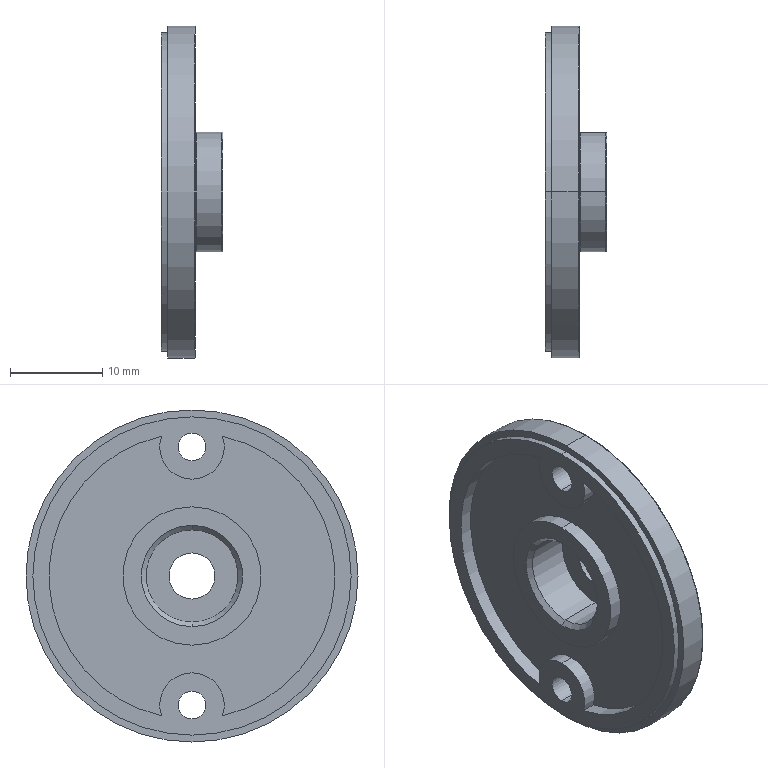Part | SolidWorks | features BaseBody 1 | 1 solid | 38 faces | box 6.7 x 36 x 36 mm | volume 2836 mm3 | cylinder 21 | plane 7 | torus 6 | cone 4 | commonest cylinder face diameters 3 x4 7 x3 5 x2 10 x2 13 x2 15 x2
STEP:
#1=CARTESIAN_POINT('',(1.5,0.,7.5));
#2=VERTEX_POINT('',#1);
#3=CARTESIAN_POINT('',(1.5,0.,-7.5));
#4=VERTEX_POINT('',#3);
#5=CARTESIAN_POINT('',(1.5,0.,0.));
#6=DIRECTION('',(-1.,0.,0.));
#7=DIRECTION('',(0.,0.,1.));
#8=AXIS2_PLACEMENT_3D('',#5,#6,#7);
#9=CIRCLE('',#8,7.5);
#10=EDGE_CURVE('',#2,#4,#9,.T.);
#11=ORIENTED_EDGE('',*,*,#10,.F.);
#12=CARTESIAN_POINT('',(1.5,0.,0.));
#13=DIRECTION('',(-1.,0.,0.));
#14=DIRECTION('',(0.,0.,1.));
#15=AXIS2_PLACEMENT_3D('',#12,#13,#14);
#16=CIRCLE('',#15,7.5);
#17=EDGE_CURVE('',#4,#2,#16,.T.);
#18=ORIENTED_EDGE('',*,*,#17,.F.);
#19=EDGE_LOOP('',(#11,#18));
#20=FACE_BOUND('',#19,.T.);
#21=CARTESIAN_POINT('',(1.5,3.308,15.143));
#22=VERTEX_POINT('',#21);
#23=CARTESIAN_POINT('',(1.5,-3.308,15.143));
#24=VERTEX_POINT('',#23);
#25=CARTESIAN_POINT('',(1.5,0.,14.));
#26=DIRECTION('',(-1.,0.,0.));
#27=DIRECTION('',(0.,0.,1.));
#28=AXIS2_PLACEMENT_3D('',#25,#26,#27);
#29=CIRCLE('',#28,3.5);
#30=EDGE_CURVE('',#22,#24,#29,.T.);
#31=ORIENTED_EDGE('',*,*,#30,.F.);
#32=CARTESIAN_POINT('',(1.5,3.308,-15.143));
#33=VERTEX_POINT('',#32);
#34=CARTESIAN_POINT('',(1.5,0.,0.));
#35=DIRECTION('',(-1.,0.,0.));
#36=DIRECTION('',(0.,0.,1.));
#37=AXIS2_PLACEMENT_3D('',#34,#35,#36);
#38=CIRCLE('',#37,15.5);
#39=EDGE_CURVE('',#22,#33,#38,.T.);
#40=ORIENTED_EDGE('',*,*,#39,.T.);
#41=CARTESIAN_POINT('',(1.5,0.,-10.5));
#42=VERTEX_POINT('',#41);
#43=CARTESIAN_POINT('',(1.5,0.,-14.));
#44=DIRECTION('',(-1.,0.,0.));
#45=DIRECTION('',(0.,0.,1.));
#46=AXIS2_PLACEMENT_3D('',#43,#44,#45);
#47=CIRCLE('',#46,3.5);
#48=EDGE_CURVE('',#42,#33,#47,.T.);
#49=ORIENTED_EDGE('',*,*,#48,.F.);
#50=CARTESIAN_POINT('',(1.5,-3.308,-15.143));
#51=VERTEX_POINT('',#50);
#52=CARTESIAN_POINT('',(1.5,0.,-14.));
#53=DIRECTION('',(-1.,0.,0.));
#54=DIRECTION('',(0.,0.,1.));
#55=AXIS2_PLACEMENT_3D('',#52,#53,#54);
#56=CIRCLE('',#55,3.5);
#57=EDGE_CURVE('',#51,#42,#56,.T.);
#58=ORIENTED_EDGE('',*,*,#57,.F.);
#59=CARTESIAN_POINT('',(1.5,0.,0.));
#60=DIRECTION('',(-1.,0.,0.));
#61=DIRECTION('',(0.,0.,1.));
#62=AXIS2_PLACEMENT_3D('',#59,#60,#61);
#63=CIRCLE('',#62,15.5);
#64=EDGE_CURVE('',#51,#24,#63,.T.);
#65=ORIENTED_EDGE('',*,*,#64,.T.);
#66=EDGE_LOOP('',(#31,#40,#49,#58,#65));
#67=FACE_OUTER_BOUND('',#66,.T.);
#68=CARTESIAN_POINT('',(1.5,0.,0.));
#69=DIRECTION('',(-1.,0.,0.));
#70=DIRECTION('',(0.,0.,1.));
#71=AXIS2_PLACEMENT_3D('',#68,#69,#70);
#72=PLANE('',#71);
#73=ADVANCED_FACE('',(#20,#67),#72,.T.);
#74=CARTESIAN_POINT('',(0.,3.308,15.143));
#75=VERTEX_POINT('',#74);
#76=CARTESIAN_POINT('',(0.,3.308,-15.143));
#77=VERTEX_POINT('',#76);
#78=CARTESIAN_POINT('',(0.,0.,0.));
#79=DIRECTION('',(-1.,0.,0.));
#80=DIRECTION('',(0.,0.,1.));
#81=AXIS2_PLACEMENT_3D('',#78,#79,#80);
#82=CIRCLE('',#81,15.5);
#83=EDGE_CURVE('',#75,#77,#82,.T.);
#84=ORIENTED_EDGE('',*,*,#83,.T.);
#85=CARTESIAN_POINT('',(1.5,3.308,-15.143));
#86=DIRECTION('',(-1.,0.,0.));
#87=VECTOR('',#86,1000.);
#88=LINE('',#85,#87);
#89=EDGE_CURVE('',#33,#77,#88,.T.);
#90=ORIENTED_EDGE('',*,*,#89,.F.);
#91=ORIENTED_EDGE('',*,*,#39,.F.);
#92=CARTESIAN_POINT('',(1.5,3.308,15.143));
#93=DIRECTION('',(-1.,0.,0.));
#94=VECTOR('',#93,1000.);
#95=LINE('',#92,#94);
#96=EDGE_CURVE('',#22,#75,#95,.T.);
#97=ORIENTED_EDGE('',*,*,#96,.T.);
#98=EDGE_LOOP('',(#84,#90,#91,#97));
#99=FACE_OUTER_BOUND('',#98,.T.);
#100=CARTESIAN_POINT('',(1.5,0.,0.));
#101=DIRECTION('',(-1.,0.,0.));
#102=DIRECTION('',(0.,0.,1.));
#103=AXIS2_PLACEMENT_3D('',#100,#101,#102);
#104=CYLINDRICAL_SURFACE('',#103,15.5);
#105=ADVANCED_FACE('',(#99),#104,.F.);
#106=CARTESIAN_POINT('',(0.,0.,-7.5));
#107=VERTEX_POINT('',#106);
#108=CARTESIAN_POINT('',(1.5,0.,-7.5));
#109=DIRECTION('',(-1.,0.,0.));
#110=VECTOR('',#109,1000.);
#111=LINE('',#108,#110);
#112=EDGE_CURVE('',#4,#107,#111,.T.);
#113=ORIENTED_EDGE('',*,*,#112,.F.);
#114=ORIENTED_EDGE('',*,*,#17,.T.);
#115=CARTESIAN_POINT('',(0.,0.,7.5));
#116=VERTEX_POINT('',#115);
#117=CARTESIAN_POINT('',(1.5,0.,7.5));
#118=DIRECTION('',(-1.,0.,0.));
#119=VECTOR('',#118,1000.);
#120=LINE('',#117,#119);
#121=EDGE_CURVE('',#2,#116,#120,.T.);
#122=ORIENTED_EDGE('',*,*,#121,.T.);
#123=CARTESIAN_POINT('',(0.,0.,0.));
#124=DIRECTION('',(-1.,0.,0.));
#125=DIRECTION('',(0.,0.,1.));
#126=AXIS2_PLACEMENT_3D('',#123,#124,#125);
#127=CIRCLE('',#126,7.5);
#128=EDGE_CURVE('',#107,#116,#127,.T.);
#129=ORIENTED_EDGE('',*,*,#128,.F.);
#130=EDGE_LOOP('',(#113,#114,#122,#129));
#131=FACE_OUTER_BOUND('',#130,.T.);
#132=CARTESIAN_POINT('',(1.5,0.,0.));
#133=DIRECTION('',(-1.,0.,0.));
#134=DIRECTION('',(0.,0.,1.));
#135=AXIS2_PLACEMENT_3D('',#132,#133,#134);
#136=CYLINDRICAL_SURFACE('',#135,7.5);
#137=ADVANCED_FACE('',(#131),#136,.T.);
#138=CARTESIAN_POINT('',(0.,0.,-10.5));
#139=VERTEX_POINT('',#138);
#140=CARTESIAN_POINT('',(1.5,0.,-10.5));
#141=DIRECTION('',(-1.,0.,0.));
#142=VECTOR('',#141,1000.);
#143=LINE('',#140,#142);
#144=EDGE_CURVE('',#42,#139,#143,.T.);
#145=ORIENTED_EDGE('',*,*,#144,.F.);
#146=ORIENTED_EDGE('',*,*,#48,.T.);
#147=ORIENTED_EDGE('',*,*,#89,.T.);
#148=CARTESIAN_POINT('',(0.,0.,-14.));
#149=DIRECTION('',(-1.,0.,0.));
#150=DIRECTION('',(0.,0.,1.));
#151=AXIS2_PLACEMENT_3D('',#148,#149,#150);
#152=CIRCLE('',#151,3.5);
#153=EDGE_CURVE('',#139,#77,#152,.T.);
#154=ORIENTED_EDGE('',*,*,#153,.F.);
#155=EDGE_LOOP('',(#145,#146,#147,#154));
#156=FACE_OUTER_BOUND('',#155,.T.);
#157=CARTESIAN_POINT('',(1.5,0.,-14.));
#158=DIRECTION('',(-1.,0.,0.));
#159=DIRECTION('',(0.,0.,1.));
#160=AXIS2_PLACEMENT_3D('',#157,#158,#159);
#161=CYLINDRICAL_SURFACE('',#160,3.5);
#162=ADVANCED_FACE('',(#156),#161,.T.);
#163=CARTESIAN_POINT('',(0.,-3.308,-15.143));
#164=VERTEX_POINT('',#163);
#165=CARTESIAN_POINT('',(0.,-3.308,15.143));
#166=VERTEX_POINT('',#165);
#167=CARTESIAN_POINT('',(0.,0.,0.));
#168=DIRECTION('',(-1.,0.,0.));
#169=DIRECTION('',(0.,0.,1.));
#170=AXIS2_PLACEMENT_3D('',#167,#168,#169);
#171=CIRCLE('',#170,15.5);
#172=EDGE_CURVE('',#164,#166,#171,.T.);
#173=ORIENTED_EDGE('',*,*,#172,.T.);
#174=CARTESIAN_POINT('',(1.5,-3.308,15.143));
#175=DIRECTION('',(-1.,0.,0.));
#176=VECTOR('',#175,1000.);
#177=LINE('',#174,#176);
#178=EDGE_CURVE('',#24,#166,#177,.T.);
#179=ORIENTED_EDGE('',*,*,#178,.F.);
#180=ORIENTED_EDGE('',*,*,#64,.F.);
#181=CARTESIAN_POINT('',(1.5,-3.308,-15.143));
#182=DIRECTION('',(-1.,0.,0.));
#183=VECTOR('',#182,1000.);
#184=LINE('',#181,#183);
#185=EDGE_CURVE('',#51,#164,#184,.T.);
#186=ORIENTED_EDGE('',*,*,#185,.T.);
#187=EDGE_LOOP('',(#173,#179,#180,#186));
#188=FACE_OUTER_BOUND('',#187,.T.);
#189=CARTESIAN_POINT('',(1.5,0.,0.));
#190=DIRECTION('',(-1.,0.,0.));
#191=DIRECTION('',(0.,0.,1.));
#192=AXIS2_PLACEMENT_3D('',#189,#190,#191);
#193=CYLINDRICAL_SURFACE('',#192,15.5);
#194=ADVANCED_FACE('',(#188),#193,.F.);
#195=CARTESIAN_POINT('',(0.,0.,14.));
#196=DIRECTION('',(-1.,0.,0.));
#197=DIRECTION('',(0.,0.,1.));
#198=AXIS2_PLACEMENT_3D('',#195,#196,#197);
#199=CIRCLE('',#198,3.5);
#200=EDGE_CURVE('',#75,#166,#199,.T.);
#201=ORIENTED_EDGE('',*,*,#200,.F.);
#202=ORIENTED_EDGE('',*,*,#96,.F.);
#203=ORIENTED_EDGE('',*,*,#30,.T.);
#204=ORIENTED_EDGE('',*,*,#178,.T.);
#205=EDGE_LOOP('',(#201,#202,#203,#204));
#206=FACE_OUTER_BOUND('',#205,.T.);
#207=CARTESIAN_POINT('',(1.5,0.,14.));
#208=DIRECTION('',(-1.,0.,0.));
#209=DIRECTION('',(0.,0.,1.));
#210=AXIS2_PLACEMENT_3D('',#207,#208,#209);
#211=CYLINDRICAL_SURFACE('',#210,3.5);
#212=ADVANCED_FACE('',(#206),#211,.T.);
#213=CARTESIAN_POINT('',(0.5,0.,-5.));
#214=VERTEX_POINT('',#213);
#215=CARTESIAN_POINT('',(0.,0.,-5.5));
#216=VERTEX_POINT('',#215);
#217=CARTESIAN_POINT('',(0.5,0.,-5.));
#218=DIRECTION('',(-0.7071,0.,-0.7071));
#219=VECTOR('',#218,1000.);
#220=LINE('',#217,#219);
#221=EDGE_CURVE('',#214,#216,#220,.T.);
#222=ORIENTED_EDGE('',*,*,#221,.F.);
#223=CARTESIAN_POINT('',(0.5,0.,5.));
#224=VERTEX_POINT('',#223);
#225=CARTESIAN_POINT('',(0.5,0.,0.));
#226=DIRECTION('',(-1.,0.,0.));
#227=DIRECTION('',(0.,0.,-1.));
#228=AXIS2_PLACEMENT_3D('',#225,#226,#227);
#229=CIRCLE('',#228,5.);
#230=EDGE_CURVE('',#224,#214,#229,.T.);
#231=ORIENTED_EDGE('',*,*,#230,.F.);
#232=CARTESIAN_POINT('',(0.,0.,5.5));
#233=VERTEX_POINT('',#232);
#234=CARTESIAN_POINT('',(0.5,0.,5.));
#235=DIRECTION('',(-0.7071,0.,0.7071));
#236=VECTOR('',#235,1000.);
#237=LINE('',#234,#236);
#238=EDGE_CURVE('',#224,#233,#237,.T.);
#239=ORIENTED_EDGE('',*,*,#238,.T.);
#240=CARTESIAN_POINT('',(0.,0.,0.));
#241=DIRECTION('',(1.,0.,0.));
#242=DIRECTION('',(0.,0.,-1.));
#243=AXIS2_PLACEMENT_3D('',#240,#241,#242);
#244=CIRCLE('',#243,5.5);
#245=EDGE_CURVE('',#216,#233,#244,.T.);
#246=ORIENTED_EDGE('',*,*,#245,.F.);
#247=EDGE_LOOP('',(#222,#231,#239,#246));
#248=FACE_OUTER_BOUND('',#247,.T.);
#249=CARTESIAN_POINT('',(0.5,0.,0.));
#250=DIRECTION('',(-1.,0.,0.));
#251=DIRECTION('',(0.,0.,1.));
#252=AXIS2_PLACEMENT_3D('',#249,#250,#251);
#253=CONICAL_SURFACE('',#252,5.,0.7854);
#254=ADVANCED_FACE('',(#248),#253,.F.);
#255=CARTESIAN_POINT('',(6.5,0.,2.5));
#256=VERTEX_POINT('',#255);
#257=CARTESIAN_POINT('',(6.7,0.,2.7));
#258=VERTEX_POINT('',#257);
#259=CARTESIAN_POINT('',(6.5,0.,2.5));
#260=DIRECTION('',(0.7071,0.,0.7071));
#261=VECTOR('',#260,1000.);
#262=LINE('',#259,#261);
#263=EDGE_CURVE('',#256,#258,#262,.T.);
#264=ORIENTED_EDGE('',*,*,#263,.F.);
#265=CARTESIAN_POINT('',(6.5,0.,-2.5));
#266=VERTEX_POINT('',#265);
#267=CARTESIAN_POINT('',(6.5,0.,0.));
#268=DIRECTION('',(1.,0.,0.));
#269=DIRECTION('',(0.,0.,1.));
#270=AXIS2_PLACEMENT_3D('',#267,#268,#269);
#271=CIRCLE('',#270,2.5);
#272=EDGE_CURVE('',#266,#256,#271,.T.);
#273=ORIENTED_EDGE('',*,*,#272,.F.);
#274=CARTESIAN_POINT('',(6.7,0.,-2.7));
#275=VERTEX_POINT('',#274);
#276=CARTESIAN_POINT('',(6.5,0.,-2.5));
#277=DIRECTION('',(0.7071,0.,-0.7071));
#278=VECTOR('',#277,1000.);
#279=LINE('',#276,#278);
#280=EDGE_CURVE('',#266,#275,#279,.T.);
#281=ORIENTED_EDGE('',*,*,#280,.T.);
#282=CARTESIAN_POINT('',(6.7,0.,0.));
#283=DIRECTION('',(-1.,0.,0.));
#284=DIRECTION('',(0.,0.,1.));
#285=AXIS2_PLACEMENT_3D('',#282,#283,#284);
#286=CIRCLE('',#285,2.7);
#287=EDGE_CURVE('',#258,#275,#286,.T.);
#288=ORIENTED_EDGE('',*,*,#287,.F.);
#289=EDGE_LOOP('',(#264,#273,#281,#288));
#290=FACE_OUTER_BOUND('',#289,.T.);
#291=CARTESIAN_POINT('',(6.5,0.,0.));
#292=DIRECTION('',(1.,0.,0.));
#293=DIRECTION('',(0.,0.,-1.));
#294=AXIS2_PLACEMENT_3D('',#291,#292,#293);
#295=CONICAL_SURFACE('',#294,2.5,0.7854);
#296=ADVANCED_FACE('',(#290),#295,.F.);
#297=CARTESIAN_POINT('',(6.7,0.,-6.4));
#298=VERTEX_POINT('',#297);
#299=CARTESIAN_POINT('',(6.6,0.,-6.5));
#300=VERTEX_POINT('',#299);
#301=CARTESIAN_POINT('',(6.6,0.,-6.4));
#302=DIRECTION('',(0.,1.,0.));
#303=DIRECTION('',(0.,0.,1.));
#304=AXIS2_PLACEMENT_3D('',#301,#302,#303);
#305=CIRCLE('',#304,0.1);
#306=EDGE_CURVE('',#298,#300,#305,.T.);
#307=ORIENTED_EDGE('',*,*,#306,.F.);
#308=CARTESIAN_POINT('',(6.7,0.,6.4));
#309=VERTEX_POINT('',#308);
#310=CARTESIAN_POINT('',(6.7,0.,0.));
#311=DIRECTION('',(1.,0.,0.));
#312=DIRECTION('',(0.,0.,1.));
#313=AXIS2_PLACEMENT_3D('',#310,#311,#312);
#314=CIRCLE('',#313,6.4);
#315=EDGE_CURVE('',#309,#298,#314,.T.);
#316=ORIENTED_EDGE('',*,*,#315,.F.);
#317=CARTESIAN_POINT('',(6.6,0.,6.5));
#318=VERTEX_POINT('',#317);
#319=CARTESIAN_POINT('',(6.6,0.,6.4));
#320=DIRECTION('',(0.,-1.,0.));
#321=DIRECTION('',(0.,0.,-1.));
#322=AXIS2_PLACEMENT_3D('',#319,#320,#321);
#323=CIRCLE('',#322,0.1);
#324=EDGE_CURVE('',#309,#318,#323,.T.);
#325=ORIENTED_EDGE('',*,*,#324,.T.);
#326=CARTESIAN_POINT('',(6.6,0.,0.));
#327=DIRECTION('',(-1.,0.,0.));
#328=DIRECTION('',(0.,0.,1.));
#329=AXIS2_PLACEMENT_3D('',#326,#327,#328);
#330=CIRCLE('',#329,6.5);
#331=EDGE_CURVE('',#300,#318,#330,.T.);
#332=ORIENTED_EDGE('',*,*,#331,.F.);
#333=EDGE_LOOP('',(#307,#316,#325,#332));
#334=FACE_OUTER_BOUND('',#333,.T.);
#335=CARTESIAN_POINT('',(6.6,0.,0.));
#336=DIRECTION('',(-1.,0.,0.));
#337=DIRECTION('',(0.,0.,1.));
#338=AXIS2_PLACEMENT_3D('',#335,#336,#337);
#339=TOROIDAL_SURFACE('',#338,6.4,0.1);
#340=ADVANCED_FACE('',(#334),#339,.T.);
#341=CARTESIAN_POINT('',(3.7,0.,-6.6));
#342=VERTEX_POINT('',#341);
#343=CARTESIAN_POINT('',(3.8,0.,-6.5));
#344=VERTEX_POINT('',#343);
#345=CARTESIAN_POINT('',(3.8,0.,-6.6));
#346=DIRECTION('',(0.,1.,0.));
#347=DIRECTION('',(0.,0.,1.));
#348=AXIS2_PLACEMENT_3D('',#345,#346,#347);
#349=CIRCLE('',#348,0.1);
#350=EDGE_CURVE('',#342,#344,#349,.T.);
#351=ORIENTED_EDGE('',*,*,#350,.F.);
#352=CARTESIAN_POINT('',(3.7,0.,6.6));
#353=VERTEX_POINT('',#352);
#354=CARTESIAN_POINT('',(3.7,0.,0.));
#355=DIRECTION('',(-1.,0.,0.));
#356=DIRECTION('',(0.,0.,1.));
#357=AXIS2_PLACEMENT_3D('',#354,#355,#356);
#358=CIRCLE('',#357,6.6);
#359=EDGE_CURVE('',#353,#342,#358,.T.);
#360=ORIENTED_EDGE('',*,*,#359,.F.);
#361=CARTESIAN_POINT('',(3.8,0.,6.5));
#362=VERTEX_POINT('',#361);
#363=CARTESIAN_POINT('',(3.8,0.,6.6));
#364=DIRECTION('',(0.,-1.,0.));
#365=DIRECTION('',(0.,0.,-1.));
#366=AXIS2_PLACEMENT_3D('',#363,#364,#365);
#367=CIRCLE('',#366,0.1);
#368=EDGE_CURVE('',#353,#362,#367,.T.);
#369=ORIENTED_EDGE('',*,*,#368,.T.);
#370=CARTESIAN_POINT('',(3.8,0.,0.));
#371=DIRECTION('',(1.,0.,0.));
#372=DIRECTION('',(0.,0.,1.));
#373=AXIS2_PLACEMENT_3D('',#370,#371,#372);
#374=CIRCLE('',#373,6.5);
#375=EDGE_CURVE('',#344,#362,#374,.T.);
#376=ORIENTED_EDGE('',*,*,#375,.F.);
#377=EDGE_LOOP('',(#351,#360,#369,#376));
#378=FACE_OUTER_BOUND('',#377,.T.);
#379=CARTESIAN_POINT('',(3.8,0.,0.));
#380=DIRECTION('',(-1.,0.,0.));
#381=DIRECTION('',(0.,0.,1.));
#382=AXIS2_PLACEMENT_3D('',#379,#380,#381);
#383=TOROIDAL_SURFACE('',#382,6.6,0.1);
#384=ADVANCED_FACE('',(#378),#383,.F.);
#385=CARTESIAN_POINT('',(3.7,0.,-17.9));
#386=VERTEX_POINT('',#385);
#387=CARTESIAN_POINT('',(3.6,0.,-18.));
#388=VERTEX_POINT('',#387);
#389=CARTESIAN_POINT('',(3.6,0.,-17.9));
#390=DIRECTION('',(0.,1.,0.));
#391=DIRECTION('',(0.,0.,1.));
#392=AXIS2_PLACEMENT_3D('',#389,#390,#391);
#393=CIRCLE('',#392,0.1);
#394=EDGE_CURVE('',#386,#388,#393,.T.);
#395=ORIENTED_EDGE('',*,*,#394,.F.);
#396=CARTESIAN_POINT('',(3.7,0.,17.9));
#397=VERTEX_POINT('',#396);
#398=CARTESIAN_POINT('',(3.7,0.,0.));
#399=DIRECTION('',(1.,0.,0.));
#400=DIRECTION('',(0.,0.,1.));
#401=AXIS2_PLACEMENT_3D('',#398,#399,#400);
#402=CIRCLE('',#401,17.9);
#403=EDGE_CURVE('',#397,#386,#402,.T.);
#404=ORIENTED_EDGE('',*,*,#403,.F.);
#405=CARTESIAN_POINT('',(3.6,0.,18.));
#406=VERTEX_POINT('',#405);
#407=CARTESIAN_POINT('',(3.6,0.,17.9));
#408=DIRECTION('',(0.,-1.,0.));
#409=DIRECTION('',(0.,0.,-1.));
#410=AXIS2_PLACEMENT_3D('',#407,#408,#409);
#411=CIRCLE('',#410,0.1);
#412=EDGE_CURVE('',#397,#406,#411,.T.);
#413=ORIENTED_EDGE('',*,*,#412,.T.);
#414=CARTESIAN_POINT('',(3.6,0.,0.));
#415=DIRECTION('',(-1.,0.,0.));
#416=DIRECTION('',(0.,0.,1.));
#417=AXIS2_PLACEMENT_3D('',#414,#415,#416);
#418=CIRCLE('',#417,18.);
#419=EDGE_CURVE('',#388,#406,#418,.T.);
#420=ORIENTED_EDGE('',*,*,#419,.F.);
#421=EDGE_LOOP('',(#395,#404,#413,#420));
#422=FACE_OUTER_BOUND('',#421,.T.);
#423=CARTESIAN_POINT('',(3.6,0.,0.));
#424=DIRECTION('',(-1.,0.,0.));
#425=DIRECTION('',(0.,0.,1.));
#426=AXIS2_PLACEMENT_3D('',#423,#424,#425);
#427=TOROIDAL_SURFACE('',#426,17.9,0.1);
#428=ADVANCED_FACE('',(#422),#427,.T.);
#429=CARTESIAN_POINT('',(3.7,0.,-15.5));
#430=VERTEX_POINT('',#429);
#431=CARTESIAN_POINT('',(0.,0.,-15.5));
#432=VERTEX_POINT('',#431);
#433=CARTESIAN_POINT('',(6.7,0.,-15.5));
#434=DIRECTION('',(-1.,0.,0.));
#435=VECTOR('',#434,1000.);
#436=LINE('',#433,#435);
#437=EDGE_CURVE('',#430,#432,#436,.T.);
#438=ORIENTED_EDGE('',*,*,#437,.F.);
#439=CARTESIAN_POINT('',(3.7,0.,-12.5));
#440=VERTEX_POINT('',#439);
#441=CARTESIAN_POINT('',(3.7,0.,-14.));
#442=DIRECTION('',(-1.,0.,0.));
#443=DIRECTION('',(0.,0.,1.));
#444=AXIS2_PLACEMENT_3D('',#441,#442,#443);
#445=CIRCLE('',#444,1.5);
#446=EDGE_CURVE('',#440,#430,#445,.T.);
#447=ORIENTED_EDGE('',*,*,#446,.F.);
#448=CARTESIAN_POINT('',(0.,0.,-12.5));
#449=VERTEX_POINT('',#448);
#450=CARTESIAN_POINT('',(6.7,0.,-12.5));
#451=DIRECTION('',(-1.,0.,0.));
#452=VECTOR('',#451,1000.);
#453=LINE('',#450,#452);
#454=EDGE_CURVE('',#440,#449,#453,.T.);
#455=ORIENTED_EDGE('',*,*,#454,.T.);
#456=CARTESIAN_POINT('',(0.,0.,-14.));
#457=DIRECTION('',(-1.,0.,0.));
#458=DIRECTION('',(0.,0.,1.));
#459=AXIS2_PLACEMENT_3D('',#456,#457,#458);
#460=CIRCLE('',#459,1.5);
#461=EDGE_CURVE('',#449,#432,#460,.T.);
#462=ORIENTED_EDGE('',*,*,#461,.T.);
#463=EDGE_LOOP('',(#438,#447,#455,#462));
#464=FACE_OUTER_BOUND('',#463,.T.);
#465=CARTESIAN_POINT('',(6.7,0.,-14.));
#466=DIRECTION('',(-1.,0.,0.));
#467=DIRECTION('',(0.,0.,1.));
#468=AXIS2_PLACEMENT_3D('',#465,#466,#467);
#469=CYLINDRICAL_SURFACE('',#468,1.5);
#470=ADVANCED_FACE('',(#464),#469,.F.);
#471=CARTESIAN_POINT('',(3.7,0.,12.5));
#472=VERTEX_POINT('',#471);
#473=CARTESIAN_POINT('',(0.,0.,12.5));
#474=VERTEX_POINT('',#473);
#475=CARTESIAN_POINT('',(6.7,0.,12.5));
#476=DIRECTION('',(-1.,0.,0.));
#477=VECTOR('',#476,1000.);
#478=LINE('',#475,#477);
#479=EDGE_CURVE('',#472,#474,#478,.T.);
#480=ORIENTED_EDGE('',*,*,#479,.F.);
#481=CARTESIAN_POINT('',(3.7,0.,15.5));
#482=VERTEX_POINT('',#481);
#483=CARTESIAN_POINT('',(3.7,0.,14.));
#484=DIRECTION('',(-1.,0.,0.));
#485=DIRECTION('',(0.,0.,1.));
#486=AXIS2_PLACEMENT_3D('',#483,#484,#485);
#487=CIRCLE('',#486,1.5);
#488=EDGE_CURVE('',#482,#472,#487,.T.);
#489=ORIENTED_EDGE('',*,*,#488,.F.);
#490=CARTESIAN_POINT('',(0.,0.,15.5));
#491=VERTEX_POINT('',#490);
#492=CARTESIAN_POINT('',(6.7,0.,15.5));
#493=DIRECTION('',(-1.,0.,0.));
#494=VECTOR('',#493,1000.);
#495=LINE('',#492,#494);
#496=EDGE_CURVE('',#482,#491,#495,.T.);
#497=ORIENTED_EDGE('',*,*,#496,.T.);
#498=CARTESIAN_POINT('',(0.,0.,14.));
#499=DIRECTION('',(-1.,0.,0.));
#500=DIRECTION('',(0.,0.,-1.));
#501=AXIS2_PLACEMENT_3D('',#498,#499,#500);
#502=CIRCLE('',#501,1.5);
#503=EDGE_CURVE('',#491,#474,#502,.T.);
#504=ORIENTED_EDGE('',*,*,#503,.T.);
#505=EDGE_LOOP('',(#480,#489,#497,#504));
#506=FACE_OUTER_BOUND('',#505,.T.);
#507=CARTESIAN_POINT('',(6.7,0.,14.));
#508=DIRECTION('',(-1.,0.,0.));
#509=DIRECTION('',(0.,0.,1.));
#510=AXIS2_PLACEMENT_3D('',#507,#508,#509);
#511=CYLINDRICAL_SURFACE('',#510,1.5);
#512=ADVANCED_FACE('',(#506),#511,.F.);
#513=CARTESIAN_POINT('',(5.1,0.,-5.));
#514=VERTEX_POINT('',#513);
#515=CARTESIAN_POINT('',(5.1,0.,-5.));
#516=DIRECTION('',(-1.,0.,0.));
#517=VECTOR('',#516,1000.);
#518=LINE('',#515,#517);
#519=EDGE_CURVE('',#514,#214,#518,.T.);
#520=ORIENTED_EDGE('',*,*,#519,.F.);
#521=CARTESIAN_POINT('',(5.1,0.,5.));
#522=VERTEX_POINT('',#521);
#523=CARTESIAN_POINT('',(5.1,0.,0.));
#524=DIRECTION('',(-1.,0.,0.));
#525=DIRECTION('',(0.,0.,1.));
#526=AXIS2_PLACEMENT_3D('',#523,#524,#525);
#527=CIRCLE('',#526,5.);
#528=EDGE_CURVE('',#522,#514,#527,.T.);
#529=ORIENTED_EDGE('',*,*,#528,.F.);
#530=CARTESIAN_POINT('',(5.1,0.,5.));
#531=DIRECTION('',(-1.,0.,0.));
#532=VECTOR('',#531,1000.);
#533=LINE('',#530,#532);
#534=EDGE_CURVE('',#522,#224,#533,.T.);
#535=ORIENTED_EDGE('',*,*,#534,.T.);
#536=ORIENTED_EDGE('',*,*,#230,.T.);
#537=EDGE_LOOP('',(#520,#529,#535,#536));
#538=FACE_OUTER_BOUND('',#537,.T.);
#539=CARTESIAN_POINT('',(5.1,0.,0.));
#540=DIRECTION('',(-1.,0.,0.));
#541=DIRECTION('',(0.,0.,1.));
#542=AXIS2_PLACEMENT_3D('',#539,#540,#541);
#543=CYLINDRICAL_SURFACE('',#542,5.);
#544=ADVANCED_FACE('',(#538),#543,.F.);
#545=CARTESIAN_POINT('',(5.1,0.,-2.5));
#546=VERTEX_POINT('',#545);
#547=CARTESIAN_POINT('',(5.1,0.,2.5));
#548=VERTEX_POINT('',#547);
#549=CARTESIAN_POINT('',(5.1,0.,0.));
#550=DIRECTION('',(1.,0.,0.));
#551=DIRECTION('',(0.,0.,1.));
#552=AXIS2_PLACEMENT_3D('',#549,#550,#551);
#553=CIRCLE('',#552,2.5);
#554=EDGE_CURVE('',#546,#548,#553,.T.);
#555=ORIENTED_EDGE('',*,*,#554,.T.);
#556=CARTESIAN_POINT('',(5.1,0.,0.));
#557=DIRECTION('',(1.,0.,0.));
#558=DIRECTION('',(0.,0.,1.));
#559=AXIS2_PLACEMENT_3D('',#556,#557,#558);
#560=CIRCLE('',#559,2.5);
#561=EDGE_CURVE('',#548,#546,#560,.T.);
#562=ORIENTED_EDGE('',*,*,#561,.T.);
#563=EDGE_LOOP('',(#555,#562));
#564=FACE_BOUND('',#563,.T.);
#565=ORIENTED_EDGE('',*,*,#528,.T.);
#566=CARTESIAN_POINT('',(5.1,0.,0.));
#567=DIRECTION('',(-1.,0.,0.));
#568=DIRECTION('',(0.,0.,1.));
#569=AXIS2_PLACEMENT_3D('',#566,#567,#568);
#570=CIRCLE('',#569,5.);
#571=EDGE_CURVE('',#514,#522,#570,.T.);
#572=ORIENTED_EDGE('',*,*,#571,.T.);
#573=EDGE_LOOP('',(#565,#572));
#574=FACE_OUTER_BOUND('',#573,.T.);
#575=CARTESIAN_POINT('',(5.1,0.,0.));
#576=DIRECTION('',(-1.,0.,0.));
#577=DIRECTION('',(0.,0.,1.));
#578=AXIS2_PLACEMENT_3D('',#575,#576,#577);
#579=PLANE('',#578);
#580=ADVANCED_FACE('',(#564,#574),#579,.T.);
#581=CARTESIAN_POINT('',(6.7,0.,0.));
#582=DIRECTION('',(-1.,0.,0.));
#583=DIRECTION('',(0.,0.,1.));
#584=AXIS2_PLACEMENT_3D('',#581,#582,#583);
#585=CIRCLE('',#584,2.7);
#586=EDGE_CURVE('',#275,#258,#585,.T.);
#587=ORIENTED_EDGE('',*,*,#586,.T.);
#588=ORIENTED_EDGE('',*,*,#287,.T.);
#589=EDGE_LOOP('',(#587,#588));
#590=FACE_BOUND('',#589,.T.);
#591=ORIENTED_EDGE('',*,*,#315,.T.);
#592=CARTESIAN_POINT('',(6.7,0.,0.));
#593=DIRECTION('',(1.,0.,0.));
#594=DIRECTION('',(0.,0.,1.));
#595=AXIS2_PLACEMENT_3D('',#592,#593,#594);
#596=CIRCLE('',#595,6.4);
#597=EDGE_CURVE('',#298,#309,#596,.T.);
#598=ORIENTED_EDGE('',*,*,#597,.T.);
#599=EDGE_LOOP('',(#591,#598));
#600=FACE_OUTER_BOUND('',#599,.T.);
#601=CARTESIAN_POINT('',(6.7,6.5,0.));
#602=DIRECTION('',(-1.,0.,0.));
#603=DIRECTION('',(0.,0.,1.));
#604=AXIS2_PLACEMENT_3D('',#601,#602,#603);
#605=PLANE('',#604);
#606=ADVANCED_FACE('',(#590,#600),#605,.F.);
#607=CARTESIAN_POINT('',(-18.807,0.,-6.5));
#608=DIRECTION('',(-1.,0.,0.));
#609=VECTOR('',#608,1000.);
#610=LINE('',#607,#609);
#611=EDGE_CURVE('',#300,#344,#610,.T.);
#612=ORIENTED_EDGE('',*,*,#611,.F.);
#613=ORIENTED_EDGE('',*,*,#331,.T.);
#614=CARTESIAN_POINT('',(-18.807,0.,6.5));
#615=DIRECTION('',(-1.,0.,0.));
#616=VECTOR('',#615,1000.);
#617=LINE('',#614,#616);
#618=EDGE_CURVE('',#318,#362,#617,.T.);
#619=ORIENTED_EDGE('',*,*,#618,.T.);
#620=CARTESIAN_POINT('',(3.8,0.,0.));
#621=DIRECTION('',(1.,0.,0.));
#622=DIRECTION('',(0.,0.,1.));
#623=AXIS2_PLACEMENT_3D('',#620,#621,#622);
#624=CIRCLE('',#623,6.5);
#625=EDGE_CURVE('',#362,#344,#624,.T.);
#626=ORIENTED_EDGE('',*,*,#625,.T.);
#627=EDGE_LOOP('',(#612,#613,#619,#626));
#628=FACE_OUTER_BOUND('',#627,.T.);
#629=CARTESIAN_POINT('',(-18.807,0.,0.));
#630=DIRECTION('',(-1.,0.,0.));
#631=DIRECTION('',(0.,0.,1.));
#632=AXIS2_PLACEMENT_3D('',#629,#630,#631);
#633=CYLINDRICAL_SURFACE('',#632,6.5);
#634=ADVANCED_FACE('',(#628),#633,.T.);
#635=ORIENTED_EDGE('',*,*,#488,.T.);
#636=CARTESIAN_POINT('',(3.7,0.,14.));
#637=DIRECTION('',(-1.,0.,0.));
#638=DIRECTION('',(0.,0.,1.));
#639=AXIS2_PLACEMENT_3D('',#636,#637,#638);
#640=CIRCLE('',#639,1.5);
#641=EDGE_CURVE('',#472,#482,#640,.T.);
#642=ORIENTED_EDGE('',*,*,#641,.T.);
#643=EDGE_LOOP('',(#635,#642));
#644=FACE_BOUND('',#643,.T.);
#645=ORIENTED_EDGE('',*,*,#446,.T.);
#646=CARTESIAN_POINT('',(3.7,0.,-14.));
#647=DIRECTION('',(-1.,0.,0.));
#648=DIRECTION('',(0.,0.,1.));
#649=AXIS2_PLACEMENT_3D('',#646,#647,#648);
#650=CIRCLE('',#649,1.5);
#651=EDGE_CURVE('',#430,#440,#650,.T.);
#652=ORIENTED_EDGE('',*,*,#651,.T.);
#653=EDGE_LOOP('',(#645,#652));
#654=FACE_BOUND('',#653,.T.);
#655=ORIENTED_EDGE('',*,*,#359,.T.);
#656=CARTESIAN_POINT('',(3.7,0.,0.));
#657=DIRECTION('',(-1.,0.,0.));
#658=DIRECTION('',(0.,0.,1.));
#659=AXIS2_PLACEMENT_3D('',#656,#657,#658);
#660=CIRCLE('',#659,6.6);
#661=EDGE_CURVE('',#342,#353,#660,.T.);
#662=ORIENTED_EDGE('',*,*,#661,.T.);
#663=EDGE_LOOP('',(#655,#662));
#664=FACE_BOUND('',#663,.T.);
#665=ORIENTED_EDGE('',*,*,#403,.T.);
#666=CARTESIAN_POINT('',(3.7,0.,0.));
#667=DIRECTION('',(1.,0.,0.));
#668=DIRECTION('',(0.,0.,1.));
#669=AXIS2_PLACEMENT_3D('',#666,#667,#668);
#670=CIRCLE('',#669,17.9);
#671=EDGE_CURVE('',#386,#397,#670,.T.);
#672=ORIENTED_EDGE('',*,*,#671,.T.);
#673=EDGE_LOOP('',(#665,#672));
#674=FACE_OUTER_BOUND('',#673,.T.);
#675=CARTESIAN_POINT('',(3.7,18.,0.));
#676=DIRECTION('',(-1.,0.,0.));
#677=DIRECTION('',(0.,0.,1.));
#678=AXIS2_PLACEMENT_3D('',#675,#676,#677);
#679=PLANE('',#678);
#680=ADVANCED_FACE('',(#644,#654,#664,#674),#679,.F.);
#681=CARTESIAN_POINT('',(0.7,0.,-18.));
#682=VERTEX_POINT('',#681);
#683=CARTESIAN_POINT('',(-18.807,0.,-18.));
#684=DIRECTION('',(-1.,0.,0.));
#685=VECTOR('',#684,1000.);
#686=LINE('',#683,#685);
#687=EDGE_CURVE('',#388,#682,#686,.T.);
#688=ORIENTED_EDGE('',*,*,#687,.F.);
#689=ORIENTED_EDGE('',*,*,#419,.T.);
#690=CARTESIAN_POINT('',(0.7,0.,18.));
#691=VERTEX_POINT('',#690);
#692=CARTESIAN_POINT('',(-18.807,0.,18.));
#693=DIRECTION('',(-1.,0.,0.));
#694=VECTOR('',#693,1000.);
#695=LINE('',#692,#694);
#696=EDGE_CURVE('',#406,#691,#695,.T.);
#697=ORIENTED_EDGE('',*,*,#696,.T.);
#698=CARTESIAN_POINT('',(0.7,0.,0.));
#699=DIRECTION('',(-1.,0.,0.));
#700=DIRECTION('',(0.,0.,1.));
#701=AXIS2_PLACEMENT_3D('',#698,#699,#700);
#702=CIRCLE('',#701,18.);
#703=EDGE_CURVE('',#682,#691,#702,.T.);
#704=ORIENTED_EDGE('',*,*,#703,.F.);
#705=EDGE_LOOP('',(#688,#689,#697,#704));
#706=FACE_OUTER_BOUND('',#705,.T.);
#707=CARTESIAN_POINT('',(-18.807,0.,0.));
#708=DIRECTION('',(-1.,0.,0.));
#709=DIRECTION('',(0.,0.,1.));
#710=AXIS2_PLACEMENT_3D('',#707,#708,#709);
#711=CYLINDRICAL_SURFACE('',#710,18.);
#712=ADVANCED_FACE('',(#706),#711,.T.);
#713=CARTESIAN_POINT('',(0.7,0.,17.25));
#714=VERTEX_POINT('',#713);
#715=CARTESIAN_POINT('',(0.7,0.,-17.25));
#716=VERTEX_POINT('',#715);
#717=CARTESIAN_POINT('',(0.7,0.,0.));
#718=DIRECTION('',(-1.,0.,0.));
#719=DIRECTION('',(0.,0.,1.));
#720=AXIS2_PLACEMENT_3D('',#717,#718,#719);
#721=CIRCLE('',#720,17.25);
#722=EDGE_CURVE('',#714,#716,#721,.T.);
#723=ORIENTED_EDGE('',*,*,#722,.F.);
#724=CARTESIAN_POINT('',(0.7,0.,0.));
#725=DIRECTION('',(-1.,0.,0.));
#726=DIRECTION('',(0.,0.,1.));
#727=AXIS2_PLACEMENT_3D('',#724,#725,#726);
#728=CIRCLE('',#727,17.25);
#729=EDGE_CURVE('',#716,#714,#728,.T.);
#730=ORIENTED_EDGE('',*,*,#729,.F.);
#731=EDGE_LOOP('',(#723,#730));
#732=FACE_BOUND('',#731,.T.);
#733=CARTESIAN_POINT('',(0.7,0.,0.));
#734=DIRECTION('',(-1.,0.,0.));
#735=DIRECTION('',(0.,0.,1.));
#736=AXIS2_PLACEMENT_3D('',#733,#734,#735);
#737=CIRCLE('',#736,18.);
#738=EDGE_CURVE('',#691,#682,#737,.T.);
#739=ORIENTED_EDGE('',*,*,#738,.T.);
#740=ORIENTED_EDGE('',*,*,#703,.T.);
#741=EDGE_LOOP('',(#739,#740));
#742=FACE_OUTER_BOUND('',#741,.T.);
#743=CARTESIAN_POINT('',(0.7,17.25,0.));
#744=DIRECTION('',(1.,0.,0.));
#745=DIRECTION('',(0.,1.,0.));
#746=AXIS2_PLACEMENT_3D('',#743,#744,#745);
#747=PLANE('',#746);
#748=ADVANCED_FACE('',(#732,#742),#747,.F.);
#749=CARTESIAN_POINT('',(0.,0.,-17.25));
#750=VERTEX_POINT('',#749);
#751=CARTESIAN_POINT('',(-18.807,0.,-17.25));
#752=DIRECTION('',(-1.,0.,0.));
#753=VECTOR('',#752,1000.);
#754=LINE('',#751,#753);
#755=EDGE_CURVE('',#716,#750,#754,.T.);
#756=ORIENTED_EDGE('',*,*,#755,.F.);
#757=ORIENTED_EDGE('',*,*,#729,.T.);
#758=CARTESIAN_POINT('',(0.,0.,17.25));
#759=VERTEX_POINT('',#758);
#760=CARTESIAN_POINT('',(-18.807,0.,17.25));
#761=DIRECTION('',(-1.,0.,0.));
#762=VECTOR('',#761,1000.);
#763=LINE('',#760,#762);
#764=EDGE_CURVE('',#714,#759,#763,.T.);
#765=ORIENTED_EDGE('',*,*,#764,.T.);
#766=CARTESIAN_POINT('',(0.,0.,0.));
#767=DIRECTION('',(-1.,0.,0.));
#768=DIRECTION('',(0.,0.,1.));
#769=AXIS2_PLACEMENT_3D('',#766,#767,#768);
#770=CIRCLE('',#769,17.25);
#771=EDGE_CURVE('',#750,#759,#770,.T.);
#772=ORIENTED_EDGE('',*,*,#771,.F.);
#773=EDGE_LOOP('',(#756,#757,#765,#772));
#774=FACE_OUTER_BOUND('',#773,.T.);
#775=CARTESIAN_POINT('',(-18.807,0.,0.));
#776=DIRECTION('',(-1.,0.,0.));
#777=DIRECTION('',(0.,0.,1.));
#778=AXIS2_PLACEMENT_3D('',#775,#776,#777);
#779=CYLINDRICAL_SURFACE('',#778,17.25);
#780=ADVANCED_FACE('',(#774),#779,.T.);
#781=CARTESIAN_POINT('',(6.7,0.,2.5));
#782=DIRECTION('',(1.,0.,0.));
#783=VECTOR('',#782,1000.);
#784=LINE('',#781,#783);
#785=EDGE_CURVE('',#548,#256,#784,.T.);
#786=ORIENTED_EDGE('',*,*,#785,.F.);
#787=ORIENTED_EDGE('',*,*,#554,.F.);
#788=CARTESIAN_POINT('',(6.7,0.,-2.5));
#789=DIRECTION('',(1.,0.,0.));
#790=VECTOR('',#789,1000.);
#791=LINE('',#788,#790);
#792=EDGE_CURVE('',#546,#266,#791,.T.);
#793=ORIENTED_EDGE('',*,*,#792,.T.);
#794=ORIENTED_EDGE('',*,*,#272,.T.);
#795=EDGE_LOOP('',(#786,#787,#793,#794));
#796=FACE_OUTER_BOUND('',#795,.T.);
#797=CARTESIAN_POINT('',(6.7,0.,0.));
#798=DIRECTION('',(1.,0.,0.));
#799=DIRECTION('',(0.,0.,-1.));
#800=AXIS2_PLACEMENT_3D('',#797,#798,#799);
#801=CYLINDRICAL_SURFACE('',#800,2.5);
#802=ADVANCED_FACE('',(#796),#801,.F.);
#803=ORIENTED_EDGE('',*,*,#200,.T.);
#804=ORIENTED_EDGE('',*,*,#172,.F.);
#805=CARTESIAN_POINT('',(0.,0.,-14.));
#806=DIRECTION('',(-1.,0.,0.));
#807=DIRECTION('',(0.,0.,1.));
#808=AXIS2_PLACEMENT_3D('',#805,#806,#807);
#809=CIRCLE('',#808,3.5);
#810=EDGE_CURVE('',#164,#139,#809,.T.);
#811=ORIENTED_EDGE('',*,*,#810,.T.);
#812=ORIENTED_EDGE('',*,*,#153,.T.);
#813=ORIENTED_EDGE('',*,*,#83,.F.);
#814=EDGE_LOOP('',(#803,#804,#811,#812,#813));
#815=FACE_BOUND('',#814,.T.);
#816=ORIENTED_EDGE('',*,*,#461,.F.);
#817=CARTESIAN_POINT('',(0.,0.,-14.));
#818=DIRECTION('',(-1.,0.,0.));
#819=DIRECTION('',(0.,0.,1.));
#820=AXIS2_PLACEMENT_3D('',#817,#818,#819);
#821=CIRCLE('',#820,1.5);
#822=EDGE_CURVE('',#432,#449,#821,.T.);
#823=ORIENTED_EDGE('',*,*,#822,.F.);
#824=EDGE_LOOP('',(#816,#823));
#825=FACE_BOUND('',#824,.T.);
#826=ORIENTED_EDGE('',*,*,#503,.F.);
#827=CARTESIAN_POINT('',(0.,0.,14.));
#828=DIRECTION('',(-1.,0.,0.));
#829=DIRECTION('',(0.,0.,-1.));
#830=AXIS2_PLACEMENT_3D('',#827,#828,#829);
#831=CIRCLE('',#830,1.5);
#832=EDGE_CURVE('',#474,#491,#831,.T.);
#833=ORIENTED_EDGE('',*,*,#832,.F.);
#834=EDGE_LOOP('',(#826,#833));
#835=FACE_BOUND('',#834,.T.);
#836=CARTESIAN_POINT('',(0.,0.,0.));
#837=DIRECTION('',(-1.,0.,0.));
#838=DIRECTION('',(0.,0.,1.));
#839=AXIS2_PLACEMENT_3D('',#836,#837,#838);
#840=CIRCLE('',#839,17.25);
#841=EDGE_CURVE('',#759,#750,#840,.T.);
#842=ORIENTED_EDGE('',*,*,#841,.T.);
#843=ORIENTED_EDGE('',*,*,#771,.T.);
#844=EDGE_LOOP('',(#842,#843));
#845=FACE_OUTER_BOUND('',#844,.T.);
#846=CARTESIAN_POINT('',(0.,0.,0.));
#847=DIRECTION('',(1.,0.,0.));
#848=DIRECTION('',(0.,1.,0.));
#849=AXIS2_PLACEMENT_3D('',#846,#847,#848);
#850=PLANE('',#849);
#851=ADVANCED_FACE('',(#815,#825,#835,#845),#850,.F.);
#852=CARTESIAN_POINT('',(0.,0.,0.));
#853=DIRECTION('',(1.,0.,0.));
#854=DIRECTION('',(0.,0.,-1.));
#855=AXIS2_PLACEMENT_3D('',#852,#853,#854);
#856=CIRCLE('',#855,5.5);
#857=EDGE_CURVE('',#233,#216,#856,.T.);
#858=ORIENTED_EDGE('',*,*,#857,.T.);
#859=ORIENTED_EDGE('',*,*,#245,.T.);
#860=EDGE_LOOP('',(#858,#859));
#861=FACE_BOUND('',#860,.T.);
#862=CARTESIAN_POINT('',(0.,0.,0.));
#863=DIRECTION('',(-1.,0.,0.));
#864=DIRECTION('',(0.,0.,1.));
#865=AXIS2_PLACEMENT_3D('',#862,#863,#864);
#866=CIRCLE('',#865,7.5);
#867=EDGE_CURVE('',#116,#107,#866,.T.);
#868=ORIENTED_EDGE('',*,*,#867,.T.);
#869=ORIENTED_EDGE('',*,*,#128,.T.);
#870=EDGE_LOOP('',(#868,#869));
#871=FACE_OUTER_BOUND('',#870,.T.);
#872=CARTESIAN_POINT('',(0.,0.,0.));
#873=DIRECTION('',(1.,0.,0.));
#874=DIRECTION('',(0.,1.,0.));
#875=AXIS2_PLACEMENT_3D('',#872,#873,#874);
#876=PLANE('',#875);
#877=ADVANCED_FACE('',(#861,#871),#876,.F.);
#878=ORIENTED_EDGE('',*,*,#561,.F.);
#879=ORIENTED_EDGE('',*,*,#785,.T.);
#880=CARTESIAN_POINT('',(6.5,0.,0.));
#881=DIRECTION('',(1.,0.,0.));
#882=DIRECTION('',(0.,0.,1.));
#883=AXIS2_PLACEMENT_3D('',#880,#881,#882);
#884=CIRCLE('',#883,2.5);
#885=EDGE_CURVE('',#256,#266,#884,.T.);
#886=ORIENTED_EDGE('',*,*,#885,.T.);
#887=ORIENTED_EDGE('',*,*,#792,.F.);
#888=EDGE_LOOP('',(#878,#879,#886,#887));
#889=FACE_OUTER_BOUND('',#888,.T.);
#890=CARTESIAN_POINT('',(6.7,0.,0.));
#891=DIRECTION('',(1.,0.,0.));
#892=DIRECTION('',(0.,0.,-1.));
#893=AXIS2_PLACEMENT_3D('',#890,#891,#892);
#894=CYLINDRICAL_SURFACE('',#893,2.5);
#895=ADVANCED_FACE('',(#889),#894,.F.);
#896=ORIENTED_EDGE('',*,*,#722,.T.);
#897=ORIENTED_EDGE('',*,*,#755,.T.);
#898=ORIENTED_EDGE('',*,*,#841,.F.);
#899=ORIENTED_EDGE('',*,*,#764,.F.);
#900=EDGE_LOOP('',(#896,#897,#898,#899));
#901=FACE_OUTER_BOUND('',#900,.T.);
#902=CARTESIAN_POINT('',(-18.807,0.,0.));
#903=DIRECTION('',(-1.,0.,0.));
#904=DIRECTION('',(0.,0.,1.));
#905=AXIS2_PLACEMENT_3D('',#902,#903,#904);
#906=CYLINDRICAL_SURFACE('',#905,17.25);
#907=ADVANCED_FACE('',(#901),#906,.T.);
#908=CARTESIAN_POINT('',(3.6,0.,0.));
#909=DIRECTION('',(-1.,0.,0.));
#910=DIRECTION('',(0.,0.,1.));
#911=AXIS2_PLACEMENT_3D('',#908,#909,#910);
#912=CIRCLE('',#911,18.);
#913=EDGE_CURVE('',#406,#388,#912,.T.);
#914=ORIENTED_EDGE('',*,*,#913,.T.);
#915=ORIENTED_EDGE('',*,*,#687,.T.);
#916=ORIENTED_EDGE('',*,*,#738,.F.);
#917=ORIENTED_EDGE('',*,*,#696,.F.);
#918=EDGE_LOOP('',(#914,#915,#916,#917));
#919=FACE_OUTER_BOUND('',#918,.T.);
#920=CARTESIAN_POINT('',(-18.807,0.,0.));
#921=DIRECTION('',(-1.,0.,0.));
#922=DIRECTION('',(0.,0.,1.));
#923=AXIS2_PLACEMENT_3D('',#920,#921,#922);
#924=CYLINDRICAL_SURFACE('',#923,18.);
#925=ADVANCED_FACE('',(#919),#924,.T.);
#926=CARTESIAN_POINT('',(6.6,0.,0.));
#927=DIRECTION('',(-1.,0.,0.));
#928=DIRECTION('',(0.,0.,1.));
#929=AXIS2_PLACEMENT_3D('',#926,#927,#928);
#930=CIRCLE('',#929,6.5);
#931=EDGE_CURVE('',#318,#300,#930,.T.);
#932=ORIENTED_EDGE('',*,*,#931,.T.);
#933=ORIENTED_EDGE('',*,*,#611,.T.);
#934=ORIENTED_EDGE('',*,*,#375,.T.);
#935=ORIENTED_EDGE('',*,*,#618,.F.);
#936=EDGE_LOOP('',(#932,#933,#934,#935));
#937=FACE_OUTER_BOUND('',#936,.T.);
#938=CARTESIAN_POINT('',(-18.807,0.,0.));
#939=DIRECTION('',(-1.,0.,0.));
#940=DIRECTION('',(0.,0.,1.));
#941=AXIS2_PLACEMENT_3D('',#938,#939,#940);
#942=CYLINDRICAL_SURFACE('',#941,6.5);
#943=ADVANCED_FACE('',(#937),#942,.T.);
#944=ORIENTED_EDGE('',*,*,#571,.F.);
#945=ORIENTED_EDGE('',*,*,#519,.T.);
#946=CARTESIAN_POINT('',(0.5,0.,0.));
#947=DIRECTION('',(-1.,0.,0.));
#948=DIRECTION('',(0.,0.,-1.));
#949=AXIS2_PLACEMENT_3D('',#946,#947,#948);
#950=CIRCLE('',#949,5.);
#951=EDGE_CURVE('',#214,#224,#950,.T.);
#952=ORIENTED_EDGE('',*,*,#951,.T.);
#953=ORIENTED_EDGE('',*,*,#534,.F.);
#954=EDGE_LOOP('',(#944,#945,#952,#953));
#955=FACE_OUTER_BOUND('',#954,.T.);
#956=CARTESIAN_POINT('',(5.1,0.,0.));
#957=DIRECTION('',(-1.,0.,0.));
#958=DIRECTION('',(0.,0.,1.));
#959=AXIS2_PLACEMENT_3D('',#956,#957,#958);
#960=CYLINDRICAL_SURFACE('',#959,5.);
#961=ADVANCED_FACE('',(#955),#960,.F.);
#962=ORIENTED_EDGE('',*,*,#641,.F.);
#963=ORIENTED_EDGE('',*,*,#479,.T.);
#964=ORIENTED_EDGE('',*,*,#832,.T.);
#965=ORIENTED_EDGE('',*,*,#496,.F.);
#966=EDGE_LOOP('',(#962,#963,#964,#965));
#967=FACE_OUTER_BOUND('',#966,.T.);
#968=CARTESIAN_POINT('',(6.7,0.,14.));
#969=DIRECTION('',(-1.,0.,0.));
#970=DIRECTION('',(0.,0.,1.));
#971=AXIS2_PLACEMENT_3D('',#968,#969,#970);
#972=CYLINDRICAL_SURFACE('',#971,1.5);
#973=ADVANCED_FACE('',(#967),#972,.F.);
#974=ORIENTED_EDGE('',*,*,#651,.F.);
#975=ORIENTED_EDGE('',*,*,#437,.T.);
#976=ORIENTED_EDGE('',*,*,#822,.T.);
#977=ORIENTED_EDGE('',*,*,#454,.F.);
#978=EDGE_LOOP('',(#974,#975,#976,#977));
#979=FACE_OUTER_BOUND('',#978,.T.);
#980=CARTESIAN_POINT('',(6.7,0.,-14.));
#981=DIRECTION('',(-1.,0.,0.));
#982=DIRECTION('',(0.,0.,1.));
#983=AXIS2_PLACEMENT_3D('',#980,#981,#982);
#984=CYLINDRICAL_SURFACE('',#983,1.5);
#985=ADVANCED_FACE('',(#979),#984,.F.);
#986=ORIENTED_EDGE('',*,*,#671,.F.);
#987=ORIENTED_EDGE('',*,*,#394,.T.);
#988=ORIENTED_EDGE('',*,*,#913,.F.);
#989=ORIENTED_EDGE('',*,*,#412,.F.);
#990=EDGE_LOOP('',(#986,#987,#988,#989));
#991=FACE_OUTER_BOUND('',#990,.T.);
#992=CARTESIAN_POINT('',(3.6,0.,0.));
#993=DIRECTION('',(-1.,0.,0.));
#994=DIRECTION('',(0.,0.,1.));
#995=AXIS2_PLACEMENT_3D('',#992,#993,#994);
#996=TOROIDAL_SURFACE('',#995,17.9,0.1);
#997=ADVANCED_FACE('',(#991),#996,.T.);
#998=ORIENTED_EDGE('',*,*,#661,.F.);
#999=ORIENTED_EDGE('',*,*,#350,.T.);
#1000=ORIENTED_EDGE('',*,*,#625,.F.);
#1001=ORIENTED_EDGE('',*,*,#368,.F.);
#1002=EDGE_LOOP('',(#998,#999,#1000,#1001));
#1003=FACE_OUTER_BOUND('',#1002,.T.);
#1004=CARTESIAN_POINT('',(3.8,0.,0.));
#1005=DIRECTION('',(-1.,0.,0.));
#1006=DIRECTION('',(0.,0.,1.));
#1007=AXIS2_PLACEMENT_3D('',#1004,#1005,#1006);
#1008=TOROIDAL_SURFACE('',#1007,6.6,0.1);
#1009=ADVANCED_FACE('',(#1003),#1008,.F.);
#1010=ORIENTED_EDGE('',*,*,#597,.F.);
#1011=ORIENTED_EDGE('',*,*,#306,.T.);
#1012=ORIENTED_EDGE('',*,*,#931,.F.);
#1013=ORIENTED_EDGE('',*,*,#324,.F.);
#1014=EDGE_LOOP('',(#1010,#1011,#1012,#1013));
#1015=FACE_OUTER_BOUND('',#1014,.T.);
#1016=CARTESIAN_POINT('',(6.6,0.,0.));
#1017=DIRECTION('',(-1.,0.,0.));
#1018=DIRECTION('',(0.,0.,1.));
#1019=AXIS2_PLACEMENT_3D('',#1016,#1017,#1018);
#1020=TOROIDAL_SURFACE('',#1019,6.4,0.1);
#1021=ADVANCED_FACE('',(#1015),#1020,.T.);
#1022=ORIENTED_EDGE('',*,*,#885,.F.);
#1023=ORIENTED_EDGE('',*,*,#263,.T.);
#1024=ORIENTED_EDGE('',*,*,#586,.F.);
#1025=ORIENTED_EDGE('',*,*,#280,.F.);
#1026=EDGE_LOOP('',(#1022,#1023,#1024,#1025));
#1027=FACE_OUTER_BOUND('',#1026,.T.);
#1028=CARTESIAN_POINT('',(6.5,0.,0.));
#1029=DIRECTION('',(1.,0.,0.));
#1030=DIRECTION('',(0.,0.,-1.));
#1031=AXIS2_PLACEMENT_3D('',#1028,#1029,#1030);
#1032=CONICAL_SURFACE('',#1031,2.5,0.7854);
#1033=ADVANCED_FACE('',(#1027),#1032,.F.);
#1034=ORIENTED_EDGE('',*,*,#951,.F.);
#1035=ORIENTED_EDGE('',*,*,#221,.T.);
#1036=ORIENTED_EDGE('',*,*,#857,.F.);
#1037=ORIENTED_EDGE('',*,*,#238,.F.);
#1038=EDGE_LOOP('',(#1034,#1035,#1036,#1037));
#1039=FACE_OUTER_BOUND('',#1038,.T.);
#1040=CARTESIAN_POINT('',(0.5,0.,0.));
#1041=DIRECTION('',(-1.,0.,0.));
#1042=DIRECTION('',(0.,0.,1.));
#1043=AXIS2_PLACEMENT_3D('',#1040,#1041,#1042);
#1044=CONICAL_SURFACE('',#1043,5.,0.7854);
#1045=ADVANCED_FACE('',(#1039),#1044,.F.);
#1046=ORIENTED_EDGE('',*,*,#57,.T.);
#1047=ORIENTED_EDGE('',*,*,#144,.T.);
#1048=ORIENTED_EDGE('',*,*,#810,.F.);
#1049=ORIENTED_EDGE('',*,*,#185,.F.);
#1050=EDGE_LOOP('',(#1046,#1047,#1048,#1049));
#1051=FACE_OUTER_BOUND('',#1050,.T.);
#1052=CARTESIAN_POINT('',(1.5,0.,-14.));
#1053=DIRECTION('',(-1.,0.,0.));
#1054=DIRECTION('',(0.,0.,1.));
#1055=AXIS2_PLACEMENT_3D('',#1052,#1053,#1054);
#1056=CYLINDRICAL_SURFACE('',#1055,3.5);
#1057=ADVANCED_FACE('',(#1051),#1056,.T.);
#1058=ORIENTED_EDGE('',*,*,#10,.T.);
#1059=ORIENTED_EDGE('',*,*,#112,.T.);
#1060=ORIENTED_EDGE('',*,*,#867,.F.);
#1061=ORIENTED_EDGE('',*,*,#121,.F.);
#1062=EDGE_LOOP('',(#1058,#1059,#1060,#1061));
#1063=FACE_OUTER_BOUND('',#1062,.T.);
#1064=CARTESIAN_POINT('',(1.5,0.,0.));
#1065=DIRECTION('',(-1.,0.,0.));
#1066=DIRECTION('',(0.,0.,1.));
#1067=AXIS2_PLACEMENT_3D('',#1064,#1065,#1066);
#1068=CYLINDRICAL_SURFACE('',#1067,7.5);
#1069=ADVANCED_FACE('',(#1063),#1068,.T.);
#1070=CLOSED_SHELL('',(#73,#105,#137,#162,#194,#212,#254,#296,#340,#384,#428,#470,#512,#544,#580,#606,#634,#680,#712,#748,#780,#802,#851,#877,#895,#907,#925,#943,#961,#973,#985,#997,#1009,#1021,#1033,#1045,#1057,#1069));
#1071=MANIFOLD_SOLID_BREP('',#1070);
#1072=CARTESIAN_POINT('',(0.,0.,0.));
#1073=DIRECTION('',(0.,0.,1.));
#1074=DIRECTION('',(1.,0.,0.));
#1075=AXIS2_PLACEMENT_3D('',#1072,#1073,#1074);
#1076=(LENGTH_UNIT()NAMED_UNIT(*)SI_UNIT(.MILLI.,.METRE.));
#1077=UNCERTAINTY_MEASURE_WITH_UNIT(LENGTH_MEASURE(0.00001),#1076,'','');
#1078=(NAMED_UNIT(*)PLANE_ANGLE_UNIT()SI_UNIT($,.RADIAN.));
#1079=(NAMED_UNIT(*)SI_UNIT($,.STERADIAN.)SOLID_ANGLE_UNIT());
#1080=(GEOMETRIC_REPRESENTATION_CONTEXT(3)GLOBAL_UNCERTAINTY_ASSIGNED_CONTEXT((#1077))GLOBAL_UNIT_ASSIGNED_CONTEXT((#1076,#1078,#1079))REPRESENTATION_CONTEXT('',''));
#1081=ADVANCED_BREP_SHAPE_REPRESENTATION('',(#1071,#1075),#1080);